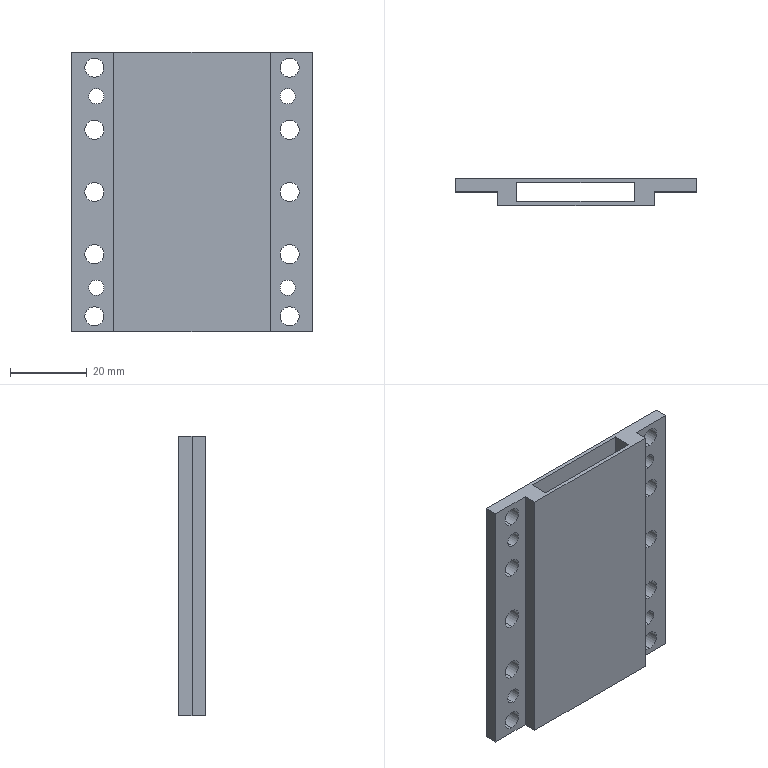Part | STEP file | Heating module 60 low | 1 solid | 42 faces | box 63 x 7 x 73 mm | volume 14494 mm3 | cylinder 28 | plane 14 | commonest cylinder face diameters 5 x20 4 x8